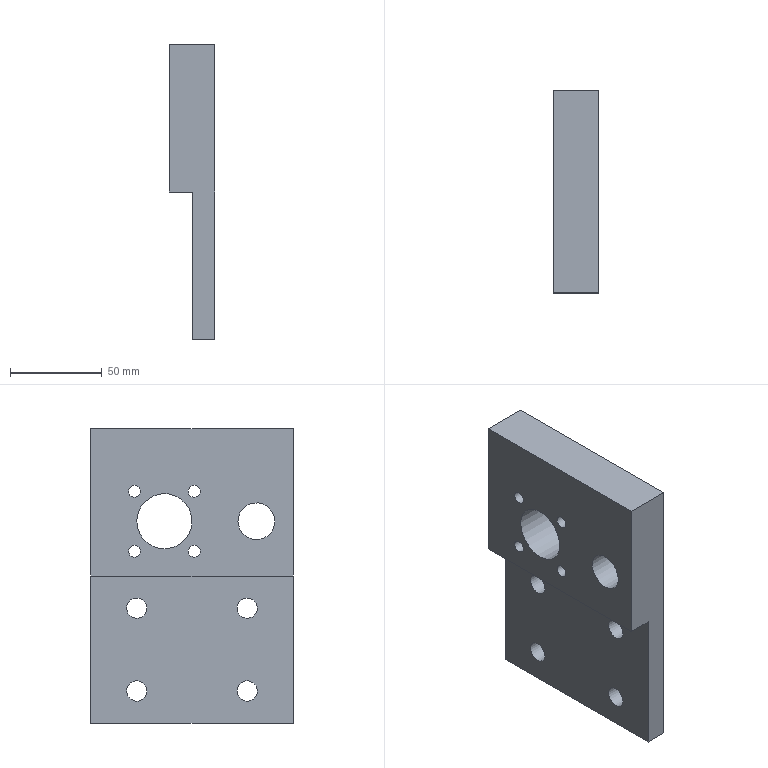Part | STEP file | SN10_015_002_PLACA | 1 solid | 18 faces | box 25 x 110 x 160 mm | volume 292195 mm3 | cylinder 10 | plane 8 | commonest cylinder face diameters 6.5 x4 11 x4 20 x1 30 x1
STEP:
#1=CARTESIAN_POINT('',(0.,0.,0.));
#2=DIRECTION('',(0.,0.,1.));
#3=DIRECTION('',(1.,0.,0.));
#4=AXIS2_PLACEMENT_3D('',#1,#2,#3);
#5=CARTESIAN_POINT('',(5499.,-1590.274,24.863));
#6=VERTEX_POINT('',#5);
#7=CARTESIAN_POINT('',(5499.,-1595.101,27.5));
#8=DIRECTION('',(-1.,0.,0.));
#9=DIRECTION('',(0.,1.,0.));
#10=AXIS2_PLACEMENT_3D('',#7,#8,#9);
#11=CIRCLE('',#10,5.5);
#12=CARTESIAN_POINT('',(5498.9,-1595.101,27.5));
#13=DIRECTION('',(-1.,0.,0.));
#14=DIRECTION('',(0.,0.8776,-0.4794));
#15=AXIS2_PLACEMENT_3D('',#12,#13,#14);
#16=CYLINDRICAL_SURFACE('',#15,5.5);
#17=CARTESIAN_POINT('',(-0.5,-0.1));
#18=DIRECTION('',(1.,0.));
#19=VECTOR('',#18,1.);
#20=LINE('',#17,#19);
#21=(GEOMETRIC_REPRESENTATION_CONTEXT(2)PARAMETRIC_REPRESENTATION_CONTEXT()REPRESENTATION_CONTEXT('',''));
#22=DEFINITIONAL_REPRESENTATION('',(#20),#21);
#23=PCURVE('',#16,#22);
#24=CARTESIAN_POINT('',(5499.,0.,0.));
#25=DIRECTION('',(1.,0.,0.));
#26=DIRECTION('',(0.,0.,-1.));
#27=AXIS2_PLACEMENT_3D('',#24,#25,#26);
#28=PLANE('',#27);
#29=CARTESIAN_POINT('',(-27.5,-1589.601));
#30=CARTESIAN_POINT('',(-17.974,-1589.601));
#31=CARTESIAN_POINT('',(-22.737,-1597.851));
#32=CARTESIAN_POINT('',(-27.5,-1606.101));
#33=CARTESIAN_POINT('',(-32.263,-1597.851));
#34=CARTESIAN_POINT('',(-37.026,-1589.601));
#35=CARTESIAN_POINT('',(-27.5,-1589.601));
#36=(BOUNDED_CURVE()B_SPLINE_CURVE(2,(#29,#30,#31,#32,#33,#34,#35),.UNSPECIFIED.,.T.,.F.)B_SPLINE_CURVE_WITH_KNOTS((1,2,2,2,2,1),(-2.094,0.,2.094,4.189,6.283,8.378),.UNSPECIFIED.)CURVE()GEOMETRIC_REPRESENTATION_ITEM()RATIONAL_B_SPLINE_CURVE((1.,0.5,1.,0.5,1.,0.5,1.))REPRESENTATION_ITEM(''));
#37=(GEOMETRIC_REPRESENTATION_CONTEXT(2)PARAMETRIC_REPRESENTATION_CONTEXT()REPRESENTATION_CONTEXT('',''));
#38=DEFINITIONAL_REPRESENTATION('',(#36),#37);
#39=PCURVE('',#28,#38);
#40=SURFACE_CURVE('',#11,(#23,#39),.PCURVE_S1.);
#41=EDGE_CURVE('',#6,#6,#40,.T.);
#42=ORIENTED_EDGE('',*,*,#41,.T.);
#43=CARTESIAN_POINT('',(5487.,-1590.274,24.863));
#44=VERTEX_POINT('',#43);
#45=CARTESIAN_POINT('',(5499.,-1590.274,24.863));
#46=CARTESIAN_POINT('',(5487.,-1590.274,24.863));
#47=B_SPLINE_CURVE_WITH_KNOTS('',1,(#45,#46),.UNSPECIFIED.,.F.,.F.,(2,2),(-0.1,11.9),.PIECEWISE_BEZIER_KNOTS.);
#48=CARTESIAN_POINT('',(6.283,0.));
#49=DIRECTION('',(0.,1.));
#50=VECTOR('',#49,1.);
#51=LINE('',#48,#50);
#52=(GEOMETRIC_REPRESENTATION_CONTEXT(2)PARAMETRIC_REPRESENTATION_CONTEXT()REPRESENTATION_CONTEXT('',''));
#53=DEFINITIONAL_REPRESENTATION('',(#51),#52);
#54=PCURVE('',#16,#53);
#55=CARTESIAN_POINT('',(0.,0.));
#56=DIRECTION('',(0.,1.));
#57=VECTOR('',#56,1.);
#58=LINE('',#55,#57);
#59=(GEOMETRIC_REPRESENTATION_CONTEXT(2)PARAMETRIC_REPRESENTATION_CONTEXT()REPRESENTATION_CONTEXT('',''));
#60=DEFINITIONAL_REPRESENTATION('',(#58),#59);
#61=PCURVE('',#16,#60);
#62=SEAM_CURVE('',#47,(#54,#61),.PCURVE_S1.);
#63=EDGE_CURVE('',#6,#44,#62,.T.);
#64=ORIENTED_EDGE('',*,*,#63,.T.);
#65=CARTESIAN_POINT('',(5487.,-1595.101,27.5));
#66=DIRECTION('',(-1.,0.,0.));
#67=DIRECTION('',(0.,1.,0.));
#68=AXIS2_PLACEMENT_3D('',#65,#66,#67);
#69=CIRCLE('',#68,5.5);
#70=CARTESIAN_POINT('',(-0.5,11.9));
#71=DIRECTION('',(1.,0.));
#72=VECTOR('',#71,1.);
#73=LINE('',#70,#72);
#74=(GEOMETRIC_REPRESENTATION_CONTEXT(2)PARAMETRIC_REPRESENTATION_CONTEXT()REPRESENTATION_CONTEXT('',''));
#75=DEFINITIONAL_REPRESENTATION('',(#73),#74);
#76=PCURVE('',#16,#75);
#77=CARTESIAN_POINT('',(5487.,-1620.101,45.));
#78=DIRECTION('',(1.,0.,0.));
#79=DIRECTION('',(0.,0.,-1.));
#80=AXIS2_PLACEMENT_3D('',#77,#78,#79);
#81=PLANE('',#80);
#82=CARTESIAN_POINT('',(17.5,30.5));
#83=CARTESIAN_POINT('',(27.026,30.5));
#84=CARTESIAN_POINT('',(22.263,22.25));
#85=CARTESIAN_POINT('',(17.5,14.));
#86=CARTESIAN_POINT('',(12.737,22.25));
#87=CARTESIAN_POINT('',(7.974,30.5));
#88=CARTESIAN_POINT('',(17.5,30.5));
#89=(BOUNDED_CURVE()B_SPLINE_CURVE(2,(#82,#83,#84,#85,#86,#87,#88),.UNSPECIFIED.,.T.,.F.)B_SPLINE_CURVE_WITH_KNOTS((1,2,2,2,2,1),(-2.094,0.,2.094,4.189,6.283,8.378),.UNSPECIFIED.)CURVE()GEOMETRIC_REPRESENTATION_ITEM()RATIONAL_B_SPLINE_CURVE((1.,0.5,1.,0.5,1.,0.5,1.))REPRESENTATION_ITEM(''));
#90=(GEOMETRIC_REPRESENTATION_CONTEXT(2)PARAMETRIC_REPRESENTATION_CONTEXT()REPRESENTATION_CONTEXT('',''));
#91=DEFINITIONAL_REPRESENTATION('',(#89),#90);
#92=PCURVE('',#81,#91);
#93=SURFACE_CURVE('',#69,(#76,#92),.PCURVE_S1.);
#94=EDGE_CURVE('',#44,#44,#93,.T.);
#95=ORIENTED_EDGE('',*,*,#94,.F.);
#96=ORIENTED_EDGE('',*,*,#63,.F.);
#97=EDGE_LOOP('',(#42,#64,#95,#96));
#98=FACE_BOUND('',#97,.F.);
#99=ADVANCED_FACE('',(#98),#16,.F.);
#100=CARTESIAN_POINT('',(5487.,-1620.101,-35.));
#101=VERTEX_POINT('',#100);
#102=CARTESIAN_POINT('',(5499.,-1620.101,-35.));
#103=VERTEX_POINT('',#102);
#104=CARTESIAN_POINT('',(5487.,-1620.101,-35.));
#105=DIRECTION('',(1.,0.,0.));
#106=VECTOR('',#105,1.);
#107=LINE('',#104,#106);
#108=CARTESIAN_POINT('',(5487.,-1510.101,-35.));
#109=DIRECTION('',(0.,0.,1.));
#110=DIRECTION('',(1.,0.,0.));
#111=AXIS2_PLACEMENT_3D('',#108,#109,#110);
#112=PLANE('',#111);
#113=CARTESIAN_POINT('',(0.,-110.));
#114=DIRECTION('',(1.,0.));
#115=VECTOR('',#114,1.);
#116=LINE('',#113,#115);
#117=(GEOMETRIC_REPRESENTATION_CONTEXT(2)PARAMETRIC_REPRESENTATION_CONTEXT()REPRESENTATION_CONTEXT('',''));
#118=DEFINITIONAL_REPRESENTATION('',(#116),#117);
#119=PCURVE('',#112,#118);
#120=CARTESIAN_POINT('',(5487.,-1620.101,45.));
#121=DIRECTION('',(0.,1.,0.));
#122=DIRECTION('',(0.,0.,1.));
#123=AXIS2_PLACEMENT_3D('',#120,#121,#122);
#124=PLANE('',#123);
#125=CARTESIAN_POINT('',(-80.,0.));
#126=DIRECTION('',(0.,1.));
#127=VECTOR('',#126,1.);
#128=LINE('',#125,#127);
#129=(GEOMETRIC_REPRESENTATION_CONTEXT(2)PARAMETRIC_REPRESENTATION_CONTEXT()REPRESENTATION_CONTEXT('',''));
#130=DEFINITIONAL_REPRESENTATION('',(#128),#129);
#131=PCURVE('',#124,#130);
#132=SURFACE_CURVE('',#107,(#119,#131),.PCURVE_S1.);
#133=EDGE_CURVE('',#101,#103,#132,.T.);
#134=ORIENTED_EDGE('',*,*,#133,.F.);
#135=CARTESIAN_POINT('',(5487.,-1510.101,-35.));
#136=VERTEX_POINT('',#135);
#137=CARTESIAN_POINT('',(5487.,-1510.101,-35.));
#138=DIRECTION('',(0.,-1.,0.));
#139=VECTOR('',#138,1.);
#140=LINE('',#137,#139);
#141=CARTESIAN_POINT('',(0.,0.));
#142=DIRECTION('',(0.,-1.));
#143=VECTOR('',#142,1.);
#144=LINE('',#141,#143);
#145=(GEOMETRIC_REPRESENTATION_CONTEXT(2)PARAMETRIC_REPRESENTATION_CONTEXT()REPRESENTATION_CONTEXT('',''));
#146=DEFINITIONAL_REPRESENTATION('',(#144),#145);
#147=PCURVE('',#112,#146);
#148=CARTESIAN_POINT('',(80.,110.));
#149=DIRECTION('',(0.,-1.));
#150=VECTOR('',#149,1.);
#151=LINE('',#148,#150);
#152=(GEOMETRIC_REPRESENTATION_CONTEXT(2)PARAMETRIC_REPRESENTATION_CONTEXT()REPRESENTATION_CONTEXT('',''));
#153=DEFINITIONAL_REPRESENTATION('',(#151),#152);
#154=PCURVE('',#81,#153);
#155=SURFACE_CURVE('',#140,(#147,#154),.PCURVE_S1.);
#156=EDGE_CURVE('',#136,#101,#155,.T.);
#157=ORIENTED_EDGE('',*,*,#156,.F.);
#158=CARTESIAN_POINT('',(5499.,-1510.101,-35.));
#159=VERTEX_POINT('',#158);
#160=CARTESIAN_POINT('',(5487.,-1510.101,-35.));
#161=DIRECTION('',(1.,0.,0.));
#162=VECTOR('',#161,1.);
#163=LINE('',#160,#162);
#164=CARTESIAN_POINT('',(0.,0.));
#165=DIRECTION('',(1.,0.));
#166=VECTOR('',#165,1.);
#167=LINE('',#164,#166);
#168=(GEOMETRIC_REPRESENTATION_CONTEXT(2)PARAMETRIC_REPRESENTATION_CONTEXT()REPRESENTATION_CONTEXT('',''));
#169=DEFINITIONAL_REPRESENTATION('',(#167),#168);
#170=PCURVE('',#112,#169);
#171=CARTESIAN_POINT('',(5473.6,-1510.101,45.));
#172=DIRECTION('',(0.,-1.,0.));
#173=DIRECTION('',(0.,0.,-1.));
#174=AXIS2_PLACEMENT_3D('',#171,#172,#173);
#175=PLANE('',#174);
#176=CARTESIAN_POINT('',(80.,13.4));
#177=DIRECTION('',(0.,1.));
#178=VECTOR('',#177,1.);
#179=LINE('',#176,#178);
#180=(GEOMETRIC_REPRESENTATION_CONTEXT(2)PARAMETRIC_REPRESENTATION_CONTEXT()REPRESENTATION_CONTEXT('',''));
#181=DEFINITIONAL_REPRESENTATION('',(#179),#180);
#182=PCURVE('',#175,#181);
#183=SURFACE_CURVE('',#163,(#170,#182),.PCURVE_S1.);
#184=EDGE_CURVE('',#136,#159,#183,.T.);
#185=ORIENTED_EDGE('',*,*,#184,.T.);
#186=CARTESIAN_POINT('',(5499.,-1510.101,-35.));
#187=DIRECTION('',(0.,-1.,0.));
#188=VECTOR('',#187,1.);
#189=LINE('',#186,#188);
#190=CARTESIAN_POINT('',(12.,0.));
#191=DIRECTION('',(0.,-1.));
#192=VECTOR('',#191,1.);
#193=LINE('',#190,#192);
#194=(GEOMETRIC_REPRESENTATION_CONTEXT(2)PARAMETRIC_REPRESENTATION_CONTEXT()REPRESENTATION_CONTEXT('',''));
#195=DEFINITIONAL_REPRESENTATION('',(#193),#194);
#196=PCURVE('',#112,#195);
#197=CARTESIAN_POINT('',(35.,-1510.101));
#198=DIRECTION('',(0.,-1.));
#199=VECTOR('',#198,1.);
#200=LINE('',#197,#199);
#201=(GEOMETRIC_REPRESENTATION_CONTEXT(2)PARAMETRIC_REPRESENTATION_CONTEXT()REPRESENTATION_CONTEXT('',''));
#202=DEFINITIONAL_REPRESENTATION('',(#200),#201);
#203=PCURVE('',#28,#202);
#204=SURFACE_CURVE('',#189,(#196,#203),.PCURVE_S1.);
#205=EDGE_CURVE('',#159,#103,#204,.T.);
#206=ORIENTED_EDGE('',*,*,#205,.T.);
#207=EDGE_LOOP('',(#134,#157,#185,#206));
#208=FACE_BOUND('',#207,.T.);
#209=ADVANCED_FACE('',(#208),#112,.F.);
#210=CARTESIAN_POINT('',(5487.,-1620.101,45.));
#211=VERTEX_POINT('',#210);
#212=CARTESIAN_POINT('',(5487.,-1510.101,45.));
#213=VERTEX_POINT('',#212);
#214=CARTESIAN_POINT('',(5487.,-1620.101,45.));
#215=DIRECTION('',(0.,1.,0.));
#216=VECTOR('',#215,1.);
#217=LINE('',#214,#216);
#218=CARTESIAN_POINT('',(0.,0.));
#219=DIRECTION('',(0.,1.));
#220=VECTOR('',#219,1.);
#221=LINE('',#218,#220);
#222=(GEOMETRIC_REPRESENTATION_CONTEXT(2)PARAMETRIC_REPRESENTATION_CONTEXT()REPRESENTATION_CONTEXT('',''));
#223=DEFINITIONAL_REPRESENTATION('',(#221),#222);
#224=PCURVE('',#81,#223);
#225=CARTESIAN_POINT('',(0.,0.,45.));
#226=DIRECTION('',(0.,0.,1.));
#227=DIRECTION('',(1.,0.,0.));
#228=AXIS2_PLACEMENT_3D('',#225,#226,#227);
#229=PLANE('',#228);
#230=CARTESIAN_POINT('',(5487.,-1620.101));
#231=DIRECTION('',(0.,1.));
#232=VECTOR('',#231,1.);
#233=LINE('',#230,#232);
#234=(GEOMETRIC_REPRESENTATION_CONTEXT(2)PARAMETRIC_REPRESENTATION_CONTEXT()REPRESENTATION_CONTEXT('',''));
#235=DEFINITIONAL_REPRESENTATION('',(#233),#234);
#236=PCURVE('',#229,#235);
#237=SURFACE_CURVE('',#217,(#224,#236),.PCURVE_S1.);
#238=EDGE_CURVE('',#211,#213,#237,.T.);
#239=ORIENTED_EDGE('',*,*,#238,.T.);
#240=CARTESIAN_POINT('',(5487.,-1510.101,-35.));
#241=DIRECTION('',(0.,0.,1.));
#242=VECTOR('',#241,1.);
#243=LINE('',#240,#242);
#244=CARTESIAN_POINT('',(80.,110.));
#245=DIRECTION('',(-1.,0.));
#246=VECTOR('',#245,1.);
#247=LINE('',#244,#246);
#248=(GEOMETRIC_REPRESENTATION_CONTEXT(2)PARAMETRIC_REPRESENTATION_CONTEXT()REPRESENTATION_CONTEXT('',''));
#249=DEFINITIONAL_REPRESENTATION('',(#247),#248);
#250=PCURVE('',#81,#249);
#251=CARTESIAN_POINT('',(80.,13.4));
#252=DIRECTION('',(-1.,0.));
#253=VECTOR('',#252,1.);
#254=LINE('',#251,#253);
#255=(GEOMETRIC_REPRESENTATION_CONTEXT(2)PARAMETRIC_REPRESENTATION_CONTEXT()REPRESENTATION_CONTEXT('',''));
#256=DEFINITIONAL_REPRESENTATION('',(#254),#255);
#257=PCURVE('',#175,#256);
#258=SURFACE_CURVE('',#243,(#250,#257),.PCURVE_S1.);
#259=EDGE_CURVE('',#136,#213,#258,.T.);
#260=ORIENTED_EDGE('',*,*,#259,.F.);
#261=ORIENTED_EDGE('',*,*,#156,.T.);
#262=CARTESIAN_POINT('',(5487.,-1620.101,45.));
#263=DIRECTION('',(0.,0.,-1.));
#264=VECTOR('',#263,1.);
#265=LINE('',#262,#264);
#266=CARTESIAN_POINT('',(0.,0.));
#267=DIRECTION('',(1.,0.));
#268=VECTOR('',#267,1.);
#269=LINE('',#266,#268);
#270=(GEOMETRIC_REPRESENTATION_CONTEXT(2)PARAMETRIC_REPRESENTATION_CONTEXT()REPRESENTATION_CONTEXT('',''));
#271=DEFINITIONAL_REPRESENTATION('',(#269),#270);
#272=PCURVE('',#81,#271);
#273=CARTESIAN_POINT('',(0.,0.));
#274=DIRECTION('',(-1.,0.));
#275=VECTOR('',#274,1.);
#276=LINE('',#273,#275);
#277=(GEOMETRIC_REPRESENTATION_CONTEXT(2)PARAMETRIC_REPRESENTATION_CONTEXT()REPRESENTATION_CONTEXT('',''));
#278=DEFINITIONAL_REPRESENTATION('',(#276),#277);
#279=PCURVE('',#124,#278);
#280=SURFACE_CURVE('',#265,(#272,#279),.PCURVE_S1.);
#281=EDGE_CURVE('',#211,#101,#280,.T.);
#282=ORIENTED_EDGE('',*,*,#281,.F.);
#283=EDGE_LOOP('',(#239,#260,#261,#282));
#284=FACE_BOUND('',#283,.T.);
#285=ORIENTED_EDGE('',*,*,#94,.F.);
#286=EDGE_LOOP('',(#285));
#287=FACE_BOUND('',#286,.T.);
#288=CARTESIAN_POINT('',(5487.,-1530.274,24.863));
#289=VERTEX_POINT('',#288);
#290=CARTESIAN_POINT('',(5487.,-1535.101,27.5));
#291=DIRECTION('',(1.,0.,0.));
#292=DIRECTION('',(0.,1.,0.));
#293=AXIS2_PLACEMENT_3D('',#290,#291,#292);
#294=CIRCLE('',#293,5.5);
#295=CARTESIAN_POINT('',(17.5,85.));
#296=DIRECTION('',(0.,1.));
#297=AXIS2_PLACEMENT_2D('',#295,#296);
#298=CIRCLE('',#297,5.5);
#299=(GEOMETRIC_REPRESENTATION_CONTEXT(2)PARAMETRIC_REPRESENTATION_CONTEXT()REPRESENTATION_CONTEXT('',''));
#300=DEFINITIONAL_REPRESENTATION('',(#298),#299);
#301=PCURVE('',#81,#300);
#302=CARTESIAN_POINT('',(5498.9,-1535.101,27.5));
#303=DIRECTION('',(-1.,0.,0.));
#304=DIRECTION('',(0.,0.8776,-0.4794));
#305=AXIS2_PLACEMENT_3D('',#302,#303,#304);
#306=CYLINDRICAL_SURFACE('',#305,5.5);
#307=CARTESIAN_POINT('',(12.066,11.9));
#308=DIRECTION('',(-1.,0.));
#309=VECTOR('',#308,1.);
#310=LINE('',#307,#309);
#311=(GEOMETRIC_REPRESENTATION_CONTEXT(2)PARAMETRIC_REPRESENTATION_CONTEXT()REPRESENTATION_CONTEXT('',''));
#312=DEFINITIONAL_REPRESENTATION('',(#310),#311);
#313=PCURVE('',#306,#312);
#314=SURFACE_CURVE('',#294,(#301,#313),.PCURVE_S1.);
#315=EDGE_CURVE('',#289,#289,#314,.T.);
#316=ORIENTED_EDGE('',*,*,#315,.T.);
#317=EDGE_LOOP('',(#316));
#318=FACE_BOUND('',#317,.T.);
#319=CARTESIAN_POINT('',(5487.,-1590.274,-20.137));
#320=VERTEX_POINT('',#319);
#321=CARTESIAN_POINT('',(5487.,-1595.101,-17.5));
#322=DIRECTION('',(1.,0.,0.));
#323=DIRECTION('',(0.,1.,0.));
#324=AXIS2_PLACEMENT_3D('',#321,#322,#323);
#325=CIRCLE('',#324,5.5);
#326=CARTESIAN_POINT('',(62.5,25.));
#327=DIRECTION('',(0.,1.));
#328=AXIS2_PLACEMENT_2D('',#326,#327);
#329=CIRCLE('',#328,5.5);
#330=(GEOMETRIC_REPRESENTATION_CONTEXT(2)PARAMETRIC_REPRESENTATION_CONTEXT()REPRESENTATION_CONTEXT('',''));
#331=DEFINITIONAL_REPRESENTATION('',(#329),#330);
#332=PCURVE('',#81,#331);
#333=CARTESIAN_POINT('',(5498.9,-1595.101,-17.5));
#334=DIRECTION('',(-1.,0.,0.));
#335=DIRECTION('',(0.,0.8776,-0.4794));
#336=AXIS2_PLACEMENT_3D('',#333,#334,#335);
#337=CYLINDRICAL_SURFACE('',#336,5.5);
#338=CARTESIAN_POINT('',(12.066,11.9));
#339=DIRECTION('',(-1.,0.));
#340=VECTOR('',#339,1.);
#341=LINE('',#338,#340);
#342=(GEOMETRIC_REPRESENTATION_CONTEXT(2)PARAMETRIC_REPRESENTATION_CONTEXT()REPRESENTATION_CONTEXT('',''));
#343=DEFINITIONAL_REPRESENTATION('',(#341),#342);
#344=PCURVE('',#337,#343);
#345=SURFACE_CURVE('',#325,(#332,#344),.PCURVE_S1.);
#346=EDGE_CURVE('',#320,#320,#345,.T.);
#347=ORIENTED_EDGE('',*,*,#346,.T.);
#348=EDGE_LOOP('',(#347));
#349=FACE_BOUND('',#348,.T.);
#350=CARTESIAN_POINT('',(5487.,-1530.274,-20.137));
#351=VERTEX_POINT('',#350);
#352=CARTESIAN_POINT('',(5487.,-1535.101,-17.5));
#353=DIRECTION('',(1.,0.,0.));
#354=DIRECTION('',(0.,1.,0.));
#355=AXIS2_PLACEMENT_3D('',#352,#353,#354);
#356=CIRCLE('',#355,5.5);
#357=CARTESIAN_POINT('',(62.5,85.));
#358=DIRECTION('',(0.,1.));
#359=AXIS2_PLACEMENT_2D('',#357,#358);
#360=CIRCLE('',#359,5.5);
#361=(GEOMETRIC_REPRESENTATION_CONTEXT(2)PARAMETRIC_REPRESENTATION_CONTEXT()REPRESENTATION_CONTEXT('',''));
#362=DEFINITIONAL_REPRESENTATION('',(#360),#361);
#363=PCURVE('',#81,#362);
#364=CARTESIAN_POINT('',(5498.9,-1535.101,-17.5));
#365=DIRECTION('',(-1.,0.,0.));
#366=DIRECTION('',(0.,0.8776,-0.4794));
#367=AXIS2_PLACEMENT_3D('',#364,#365,#366);
#368=CYLINDRICAL_SURFACE('',#367,5.5);
#369=CARTESIAN_POINT('',(12.066,11.9));
#370=DIRECTION('',(-1.,0.));
#371=VECTOR('',#370,1.);
#372=LINE('',#369,#371);
#373=(GEOMETRIC_REPRESENTATION_CONTEXT(2)PARAMETRIC_REPRESENTATION_CONTEXT()REPRESENTATION_CONTEXT('',''));
#374=DEFINITIONAL_REPRESENTATION('',(#372),#373);
#375=PCURVE('',#368,#374);
#376=SURFACE_CURVE('',#356,(#363,#375),.PCURVE_S1.);
#377=EDGE_CURVE('',#351,#351,#376,.T.);
#378=ORIENTED_EDGE('',*,*,#377,.T.);
#379=EDGE_LOOP('',(#378));
#380=FACE_BOUND('',#379,.T.);
#381=ADVANCED_FACE('',(#284,#287,#318,#349,#380),#81,.F.);
#382=CARTESIAN_POINT('',(5499.,-1620.101,125.));
#383=VERTEX_POINT('',#382);
#384=CARTESIAN_POINT('',(5499.,-1620.101,125.));
#385=DIRECTION('',(0.,0.,-1.));
#386=VECTOR('',#385,1.);
#387=LINE('',#384,#386);
#388=CARTESIAN_POINT('',(-125.,-1620.101));
#389=DIRECTION('',(1.,0.));
#390=VECTOR('',#389,1.);
#391=LINE('',#388,#390);
#392=(GEOMETRIC_REPRESENTATION_CONTEXT(2)PARAMETRIC_REPRESENTATION_CONTEXT()REPRESENTATION_CONTEXT('',''));
#393=DEFINITIONAL_REPRESENTATION('',(#391),#392);
#394=PCURVE('',#28,#393);
#395=CARTESIAN_POINT('',(80.,12.));
#396=DIRECTION('',(-1.,0.));
#397=VECTOR('',#396,1.);
#398=LINE('',#395,#397);
#399=(GEOMETRIC_REPRESENTATION_CONTEXT(2)PARAMETRIC_REPRESENTATION_CONTEXT()REPRESENTATION_CONTEXT('',''));
#400=DEFINITIONAL_REPRESENTATION('',(#398),#399);
#401=PCURVE('',#124,#400);
#402=SURFACE_CURVE('',#387,(#394,#401),.PCURVE_S1.);
#403=EDGE_CURVE('',#383,#103,#402,.T.);
#404=ORIENTED_EDGE('',*,*,#403,.T.);
#405=ORIENTED_EDGE('',*,*,#205,.F.);
#406=CARTESIAN_POINT('',(5499.,-1510.101,125.));
#407=VERTEX_POINT('',#406);
#408=CARTESIAN_POINT('',(5499.,-1510.101,-35.));
#409=DIRECTION('',(0.,0.,1.));
#410=VECTOR('',#409,1.);
#411=LINE('',#408,#410);
#412=CARTESIAN_POINT('',(35.,-1510.101));
#413=DIRECTION('',(-1.,0.));
#414=VECTOR('',#413,1.);
#415=LINE('',#412,#414);
#416=(GEOMETRIC_REPRESENTATION_CONTEXT(2)PARAMETRIC_REPRESENTATION_CONTEXT()REPRESENTATION_CONTEXT('',''));
#417=DEFINITIONAL_REPRESENTATION('',(#415),#416);
#418=PCURVE('',#28,#417);
#419=CARTESIAN_POINT('',(80.,25.4));
#420=DIRECTION('',(-1.,0.));
#421=VECTOR('',#420,1.);
#422=LINE('',#419,#421);
#423=(GEOMETRIC_REPRESENTATION_CONTEXT(2)PARAMETRIC_REPRESENTATION_CONTEXT()REPRESENTATION_CONTEXT('',''));
#424=DEFINITIONAL_REPRESENTATION('',(#422),#423);
#425=PCURVE('',#175,#424);
#426=SURFACE_CURVE('',#411,(#418,#425),.PCURVE_S1.);
#427=EDGE_CURVE('',#159,#407,#426,.T.);
#428=ORIENTED_EDGE('',*,*,#427,.T.);
#429=CARTESIAN_POINT('',(5499.,-1620.101,125.));
#430=DIRECTION('',(0.,1.,0.));
#431=VECTOR('',#430,1.);
#432=LINE('',#429,#431);
#433=CARTESIAN_POINT('',(-125.,-1620.101));
#434=DIRECTION('',(0.,1.));
#435=VECTOR('',#434,1.);
#436=LINE('',#433,#435);
#437=(GEOMETRIC_REPRESENTATION_CONTEXT(2)PARAMETRIC_REPRESENTATION_CONTEXT()REPRESENTATION_CONTEXT('',''));
#438=DEFINITIONAL_REPRESENTATION('',(#436),#437);
#439=PCURVE('',#28,#438);
#440=CARTESIAN_POINT('',(0.,0.,125.));
#441=DIRECTION('',(0.,0.,1.));
#442=DIRECTION('',(1.,0.,0.));
#443=AXIS2_PLACEMENT_3D('',#440,#441,#442);
#444=PLANE('',#443);
#445=CARTESIAN_POINT('',(5499.,-1620.101));
#446=DIRECTION('',(0.,1.));
#447=VECTOR('',#446,1.);
#448=LINE('',#445,#447);
#449=(GEOMETRIC_REPRESENTATION_CONTEXT(2)PARAMETRIC_REPRESENTATION_CONTEXT()REPRESENTATION_CONTEXT('',''));
#450=DEFINITIONAL_REPRESENTATION('',(#448),#449);
#451=PCURVE('',#444,#450);
#452=SURFACE_CURVE('',#432,(#439,#451),.PCURVE_S1.);
#453=EDGE_CURVE('',#383,#407,#452,.T.);
#454=ORIENTED_EDGE('',*,*,#453,.F.);
#455=EDGE_LOOP('',(#404,#405,#428,#454));
#456=FACE_BOUND('',#455,.T.);
#457=ORIENTED_EDGE('',*,*,#41,.T.);
#458=EDGE_LOOP('',(#457));
#459=FACE_BOUND('',#458,.T.);
#460=CARTESIAN_POINT('',(5499.,-1591.325,69.956));
#461=VERTEX_POINT('',#460);
#462=CARTESIAN_POINT('',(5499.,-1600.101,74.75));
#463=DIRECTION('',(1.,0.,0.));
#464=DIRECTION('',(0.,1.,0.));
#465=AXIS2_PLACEMENT_3D('',#462,#463,#464);
#466=CIRCLE('',#465,10.);
#467=CARTESIAN_POINT('',(-74.75,-1600.101));
#468=DIRECTION('',(0.,1.));
#469=AXIS2_PLACEMENT_2D('',#467,#468);
#470=CIRCLE('',#469,10.);
#471=(GEOMETRIC_REPRESENTATION_CONTEXT(2)PARAMETRIC_REPRESENTATION_CONTEXT()REPRESENTATION_CONTEXT('',''));
#472=DEFINITIONAL_REPRESENTATION('',(#470),#471);
#473=PCURVE('',#28,#472);
#474=CARTESIAN_POINT('',(5498.9,-1600.101,74.75));
#475=DIRECTION('',(-1.,0.,0.));
#476=DIRECTION('',(0.,0.8776,-0.4794));
#477=AXIS2_PLACEMENT_3D('',#474,#475,#476);
#478=CYLINDRICAL_SURFACE('',#477,10.);
#479=CARTESIAN_POINT('',(12.066,-0.1));
#480=DIRECTION('',(-1.,0.));
#481=VECTOR('',#480,1.);
#482=LINE('',#479,#481);
#483=(GEOMETRIC_REPRESENTATION_CONTEXT(2)PARAMETRIC_REPRESENTATION_CONTEXT()REPRESENTATION_CONTEXT('',''));
#484=DEFINITIONAL_REPRESENTATION('',(#482),#483);
#485=PCURVE('',#478,#484);
#486=SURFACE_CURVE('',#466,(#473,#485),.PCURVE_S1.);
#487=EDGE_CURVE('',#461,#461,#486,.T.);
#488=ORIENTED_EDGE('',*,*,#487,.F.);
#489=EDGE_LOOP('',(#488));
#490=FACE_BOUND('',#489,.T.);
#491=CARTESIAN_POINT('',(5499.,-1569.203,89.442));
#492=VERTEX_POINT('',#491);
#493=CARTESIAN_POINT('',(5499.,-1566.351,91.));
#494=DIRECTION('',(1.,0.,0.));
#495=DIRECTION('',(0.,1.,0.));
#496=AXIS2_PLACEMENT_3D('',#493,#494,#495);
#497=CIRCLE('',#496,3.25);
#498=CARTESIAN_POINT('',(-91.,-1566.351));
#499=DIRECTION('',(0.,1.));
#500=AXIS2_PLACEMENT_2D('',#498,#499);
#501=CIRCLE('',#500,3.25);
#502=(GEOMETRIC_REPRESENTATION_CONTEXT(2)PARAMETRIC_REPRESENTATION_CONTEXT()REPRESENTATION_CONTEXT('',''));
#503=DEFINITIONAL_REPRESENTATION('',(#501),#502);
#504=PCURVE('',#28,#503);
#505=CARTESIAN_POINT('',(5473.7,-1566.351,91.));
#506=DIRECTION('',(1.,0.,0.));
#507=DIRECTION('',(0.,0.8776,0.4794));
#508=AXIS2_PLACEMENT_3D('',#505,#506,#507);
#509=CYLINDRICAL_SURFACE('',#508,3.25);
#510=CARTESIAN_POINT('',(-0.5,25.3));
#511=DIRECTION('',(1.,0.));
#512=VECTOR('',#511,1.);
#513=LINE('',#510,#512);
#514=(GEOMETRIC_REPRESENTATION_CONTEXT(2)PARAMETRIC_REPRESENTATION_CONTEXT()REPRESENTATION_CONTEXT('',''));
#515=DEFINITIONAL_REPRESENTATION('',(#513),#514);
#516=PCURVE('',#509,#515);
#517=SURFACE_CURVE('',#497,(#504,#516),.PCURVE_S1.);
#518=EDGE_CURVE('',#492,#492,#517,.T.);
#519=ORIENTED_EDGE('',*,*,#518,.F.);
#520=EDGE_LOOP('',(#519));
#521=FACE_BOUND('',#520,.T.);
#522=CARTESIAN_POINT('',(5499.,-1563.264,67.559));
#523=VERTEX_POINT('',#522);
#524=CARTESIAN_POINT('',(5499.,-1550.101,74.75));
#525=DIRECTION('',(1.,0.,0.));
#526=DIRECTION('',(0.,1.,0.));
#527=AXIS2_PLACEMENT_3D('',#524,#525,#526);
#528=CIRCLE('',#527,15.);
#529=CARTESIAN_POINT('',(-74.75,-1550.101));
#530=DIRECTION('',(0.,1.));
#531=AXIS2_PLACEMENT_2D('',#529,#530);
#532=CIRCLE('',#531,15.);
#533=(GEOMETRIC_REPRESENTATION_CONTEXT(2)PARAMETRIC_REPRESENTATION_CONTEXT()REPRESENTATION_CONTEXT('',''));
#534=DEFINITIONAL_REPRESENTATION('',(#532),#533);
#535=PCURVE('',#28,#534);
#536=CARTESIAN_POINT('',(5473.7,-1550.101,74.75));
#537=DIRECTION('',(1.,0.,0.));
#538=DIRECTION('',(0.,0.8776,0.4794));
#539=AXIS2_PLACEMENT_3D('',#536,#537,#538);
#540=CYLINDRICAL_SURFACE('',#539,15.);
#541=CARTESIAN_POINT('',(-0.5,25.3));
#542=DIRECTION('',(1.,0.));
#543=VECTOR('',#542,1.);
#544=LINE('',#541,#543);
#545=(GEOMETRIC_REPRESENTATION_CONTEXT(2)PARAMETRIC_REPRESENTATION_CONTEXT()REPRESENTATION_CONTEXT('',''));
#546=DEFINITIONAL_REPRESENTATION('',(#544),#545);
#547=PCURVE('',#540,#546);
#548=SURFACE_CURVE('',#528,(#535,#547),.PCURVE_S1.);
#549=EDGE_CURVE('',#523,#523,#548,.T.);
#550=ORIENTED_EDGE('',*,*,#549,.F.);
#551=EDGE_LOOP('',(#550));
#552=FACE_BOUND('',#551,.T.);
#553=CARTESIAN_POINT('',(5499.,-1530.998,92.558));
#554=VERTEX_POINT('',#553);
#555=CARTESIAN_POINT('',(5499.,-1533.851,91.));
#556=DIRECTION('',(1.,0.,0.));
#557=DIRECTION('',(0.,1.,0.));
#558=AXIS2_PLACEMENT_3D('',#555,#556,#557);
#559=CIRCLE('',#558,3.25);
#560=CARTESIAN_POINT('',(-91.,-1533.851));
#561=DIRECTION('',(0.,1.));
#562=AXIS2_PLACEMENT_2D('',#560,#561);
#563=CIRCLE('',#562,3.25);
#564=(GEOMETRIC_REPRESENTATION_CONTEXT(2)PARAMETRIC_REPRESENTATION_CONTEXT()REPRESENTATION_CONTEXT('',''));
#565=DEFINITIONAL_REPRESENTATION('',(#563),#564);
#566=PCURVE('',#28,#565);
#567=CARTESIAN_POINT('',(5473.7,-1533.851,91.));
#568=DIRECTION('',(1.,0.,0.));
#569=DIRECTION('',(0.,0.8776,0.4794));
#570=AXIS2_PLACEMENT_3D('',#567,#568,#569);
#571=CYLINDRICAL_SURFACE('',#570,3.25);
#572=CARTESIAN_POINT('',(-0.5,25.3));
#573=DIRECTION('',(1.,0.));
#574=VECTOR('',#573,1.);
#575=LINE('',#572,#574);
#576=(GEOMETRIC_REPRESENTATION_CONTEXT(2)PARAMETRIC_REPRESENTATION_CONTEXT()REPRESENTATION_CONTEXT('',''));
#577=DEFINITIONAL_REPRESENTATION('',(#575),#576);
#578=PCURVE('',#571,#577);
#579=SURFACE_CURVE('',#559,(#566,#578),.PCURVE_S1.);
#580=EDGE_CURVE('',#554,#554,#579,.T.);
#581=ORIENTED_EDGE('',*,*,#580,.F.);
#582=EDGE_LOOP('',(#581));
#583=FACE_BOUND('',#582,.T.);
#584=CARTESIAN_POINT('',(5499.,-1563.498,60.058));
#585=VERTEX_POINT('',#584);
#586=CARTESIAN_POINT('',(5499.,-1566.351,58.5));
#587=DIRECTION('',(1.,0.,0.));
#588=DIRECTION('',(0.,1.,0.));
#589=AXIS2_PLACEMENT_3D('',#586,#587,#588);
#590=CIRCLE('',#589,3.25);
#591=CARTESIAN_POINT('',(-58.5,-1566.351));
#592=DIRECTION('',(0.,1.));
#593=AXIS2_PLACEMENT_2D('',#591,#592);
#594=CIRCLE('',#593,3.25);
#595=(GEOMETRIC_REPRESENTATION_CONTEXT(2)PARAMETRIC_REPRESENTATION_CONTEXT()REPRESENTATION_CONTEXT('',''));
#596=DEFINITIONAL_REPRESENTATION('',(#594),#595);
#597=PCURVE('',#28,#596);
#598=CARTESIAN_POINT('',(5473.7,-1566.351,58.5));
#599=DIRECTION('',(1.,0.,0.));
#600=DIRECTION('',(0.,0.8776,0.4794));
#601=AXIS2_PLACEMENT_3D('',#598,#599,#600);
#602=CYLINDRICAL_SURFACE('',#601,3.25);
#603=CARTESIAN_POINT('',(-0.5,25.3));
#604=DIRECTION('',(1.,0.));
#605=VECTOR('',#604,1.);
#606=LINE('',#603,#605);
#607=(GEOMETRIC_REPRESENTATION_CONTEXT(2)PARAMETRIC_REPRESENTATION_CONTEXT()REPRESENTATION_CONTEXT('',''));
#608=DEFINITIONAL_REPRESENTATION('',(#606),#607);
#609=PCURVE('',#602,#608);
#610=SURFACE_CURVE('',#590,(#597,#609),.PCURVE_S1.);
#611=EDGE_CURVE('',#585,#585,#610,.T.);
#612=ORIENTED_EDGE('',*,*,#611,.F.);
#613=EDGE_LOOP('',(#612));
#614=FACE_BOUND('',#613,.T.);
#615=CARTESIAN_POINT('',(5499.,-1530.998,60.058));
#616=VERTEX_POINT('',#615);
#617=CARTESIAN_POINT('',(5499.,-1533.851,58.5));
#618=DIRECTION('',(1.,0.,0.));
#619=DIRECTION('',(0.,1.,0.));
#620=AXIS2_PLACEMENT_3D('',#617,#618,#619);
#621=CIRCLE('',#620,3.25);
#622=CARTESIAN_POINT('',(-58.5,-1533.851));
#623=DIRECTION('',(0.,1.));
#624=AXIS2_PLACEMENT_2D('',#622,#623);
#625=CIRCLE('',#624,3.25);
#626=(GEOMETRIC_REPRESENTATION_CONTEXT(2)PARAMETRIC_REPRESENTATION_CONTEXT()REPRESENTATION_CONTEXT('',''));
#627=DEFINITIONAL_REPRESENTATION('',(#625),#626);
#628=PCURVE('',#28,#627);
#629=CARTESIAN_POINT('',(5473.7,-1533.851,58.5));
#630=DIRECTION('',(1.,0.,0.));
#631=DIRECTION('',(0.,0.8776,0.4794));
#632=AXIS2_PLACEMENT_3D('',#629,#630,#631);
#633=CYLINDRICAL_SURFACE('',#632,3.25);
#634=CARTESIAN_POINT('',(-0.5,25.3));
#635=DIRECTION('',(1.,0.));
#636=VECTOR('',#635,1.);
#637=LINE('',#634,#636);
#638=(GEOMETRIC_REPRESENTATION_CONTEXT(2)PARAMETRIC_REPRESENTATION_CONTEXT()REPRESENTATION_CONTEXT('',''));
#639=DEFINITIONAL_REPRESENTATION('',(#637),#638);
#640=PCURVE('',#633,#639);
#641=SURFACE_CURVE('',#621,(#628,#640),.PCURVE_S1.);
#642=EDGE_CURVE('',#616,#616,#641,.T.);
#643=ORIENTED_EDGE('',*,*,#642,.F.);
#644=EDGE_LOOP('',(#643));
#645=FACE_BOUND('',#644,.T.);
#646=CARTESIAN_POINT('',(5499.,-1530.274,24.863));
#647=VERTEX_POINT('',#646);
#648=CARTESIAN_POINT('',(5499.,-1535.101,27.5));
#649=DIRECTION('',(1.,0.,0.));
#650=DIRECTION('',(0.,1.,0.));
#651=AXIS2_PLACEMENT_3D('',#648,#649,#650);
#652=CIRCLE('',#651,5.5);
#653=CARTESIAN_POINT('',(-27.5,-1535.101));
#654=DIRECTION('',(0.,1.));
#655=AXIS2_PLACEMENT_2D('',#653,#654);
#656=CIRCLE('',#655,5.5);
#657=(GEOMETRIC_REPRESENTATION_CONTEXT(2)PARAMETRIC_REPRESENTATION_CONTEXT()REPRESENTATION_CONTEXT('',''));
#658=DEFINITIONAL_REPRESENTATION('',(#656),#657);
#659=PCURVE('',#28,#658);
#660=CARTESIAN_POINT('',(12.066,-0.1));
#661=DIRECTION('',(-1.,0.));
#662=VECTOR('',#661,1.);
#663=LINE('',#660,#662);
#664=(GEOMETRIC_REPRESENTATION_CONTEXT(2)PARAMETRIC_REPRESENTATION_CONTEXT()REPRESENTATION_CONTEXT('',''));
#665=DEFINITIONAL_REPRESENTATION('',(#663),#664);
#666=PCURVE('',#306,#665);
#667=SURFACE_CURVE('',#652,(#659,#666),.PCURVE_S1.);
#668=EDGE_CURVE('',#647,#647,#667,.T.);
#669=ORIENTED_EDGE('',*,*,#668,.F.);
#670=EDGE_LOOP('',(#669));
#671=FACE_BOUND('',#670,.T.);
#672=CARTESIAN_POINT('',(5499.,-1590.274,-20.137));
#673=VERTEX_POINT('',#672);
#674=CARTESIAN_POINT('',(5499.,-1595.101,-17.5));
#675=DIRECTION('',(1.,0.,0.));
#676=DIRECTION('',(0.,1.,0.));
#677=AXIS2_PLACEMENT_3D('',#674,#675,#676);
#678=CIRCLE('',#677,5.5);
#679=CARTESIAN_POINT('',(17.5,-1595.101));
#680=DIRECTION('',(0.,1.));
#681=AXIS2_PLACEMENT_2D('',#679,#680);
#682=CIRCLE('',#681,5.5);
#683=(GEOMETRIC_REPRESENTATION_CONTEXT(2)PARAMETRIC_REPRESENTATION_CONTEXT()REPRESENTATION_CONTEXT('',''));
#684=DEFINITIONAL_REPRESENTATION('',(#682),#683);
#685=PCURVE('',#28,#684);
#686=CARTESIAN_POINT('',(12.066,-0.1));
#687=DIRECTION('',(-1.,0.));
#688=VECTOR('',#687,1.);
#689=LINE('',#686,#688);
#690=(GEOMETRIC_REPRESENTATION_CONTEXT(2)PARAMETRIC_REPRESENTATION_CONTEXT()REPRESENTATION_CONTEXT('',''));
#691=DEFINITIONAL_REPRESENTATION('',(#689),#690);
#692=PCURVE('',#337,#691);
#693=SURFACE_CURVE('',#678,(#685,#692),.PCURVE_S1.);
#694=EDGE_CURVE('',#673,#673,#693,.T.);
#695=ORIENTED_EDGE('',*,*,#694,.F.);
#696=EDGE_LOOP('',(#695));
#697=FACE_BOUND('',#696,.T.);
#698=CARTESIAN_POINT('',(5499.,-1530.274,-20.137));
#699=VERTEX_POINT('',#698);
#700=CARTESIAN_POINT('',(5499.,-1535.101,-17.5));
#701=DIRECTION('',(1.,0.,0.));
#702=DIRECTION('',(0.,1.,0.));
#703=AXIS2_PLACEMENT_3D('',#700,#701,#702);
#704=CIRCLE('',#703,5.5);
#705=CARTESIAN_POINT('',(17.5,-1535.101));
#706=DIRECTION('',(0.,1.));
#707=AXIS2_PLACEMENT_2D('',#705,#706);
#708=CIRCLE('',#707,5.5);
#709=(GEOMETRIC_REPRESENTATION_CONTEXT(2)PARAMETRIC_REPRESENTATION_CONTEXT()REPRESENTATION_CONTEXT('',''));
#710=DEFINITIONAL_REPRESENTATION('',(#708),#709);
#711=PCURVE('',#28,#710);
#712=CARTESIAN_POINT('',(12.066,-0.1));
#713=DIRECTION('',(-1.,0.));
#714=VECTOR('',#713,1.);
#715=LINE('',#712,#714);
#716=(GEOMETRIC_REPRESENTATION_CONTEXT(2)PARAMETRIC_REPRESENTATION_CONTEXT()REPRESENTATION_CONTEXT('',''));
#717=DEFINITIONAL_REPRESENTATION('',(#715),#716);
#718=PCURVE('',#368,#717);
#719=SURFACE_CURVE('',#704,(#711,#718),.PCURVE_S1.);
#720=EDGE_CURVE('',#699,#699,#719,.T.);
#721=ORIENTED_EDGE('',*,*,#720,.F.);
#722=EDGE_LOOP('',(#721));
#723=FACE_BOUND('',#722,.T.);
#724=ADVANCED_FACE('',(#456,#459,#490,#521,#552,#583,#614,#645,#671,#697,#723),#28,.T.);
#725=ORIENTED_EDGE('',*,*,#720,.F.);
#726=CARTESIAN_POINT('',(5499.,-1530.274,-20.137));
#727=CARTESIAN_POINT('',(5487.,-1530.274,-20.137));
#728=B_SPLINE_CURVE_WITH_KNOTS('',1,(#726,#727),.UNSPECIFIED.,.F.,.F.,(2,2),(-0.1,11.9),.PIECEWISE_BEZIER_KNOTS.);
#729=CARTESIAN_POINT('',(6.283,0.));
#730=DIRECTION('',(0.,1.));
#731=VECTOR('',#730,1.);
#732=LINE('',#729,#731);
#733=(GEOMETRIC_REPRESENTATION_CONTEXT(2)PARAMETRIC_REPRESENTATION_CONTEXT()REPRESENTATION_CONTEXT('',''));
#734=DEFINITIONAL_REPRESENTATION('',(#732),#733);
#735=PCURVE('',#368,#734);
#736=CARTESIAN_POINT('',(0.,0.));
#737=DIRECTION('',(0.,1.));
#738=VECTOR('',#737,1.);
#739=LINE('',#736,#738);
#740=(GEOMETRIC_REPRESENTATION_CONTEXT(2)PARAMETRIC_REPRESENTATION_CONTEXT()REPRESENTATION_CONTEXT('',''));
#741=DEFINITIONAL_REPRESENTATION('',(#739),#740);
#742=PCURVE('',#368,#741);
#743=SEAM_CURVE('',#728,(#735,#742),.PCURVE_S1.);
#744=EDGE_CURVE('',#699,#351,#743,.T.);
#745=ORIENTED_EDGE('',*,*,#744,.T.);
#746=ORIENTED_EDGE('',*,*,#377,.T.);
#747=ORIENTED_EDGE('',*,*,#744,.F.);
#748=EDGE_LOOP('',(#725,#745,#746,#747));
#749=FACE_BOUND('',#748,.F.);
#750=ADVANCED_FACE('',(#749),#368,.F.);
#751=ORIENTED_EDGE('',*,*,#694,.F.);
#752=CARTESIAN_POINT('',(5499.,-1590.274,-20.137));
#753=CARTESIAN_POINT('',(5487.,-1590.274,-20.137));
#754=B_SPLINE_CURVE_WITH_KNOTS('',1,(#752,#753),.UNSPECIFIED.,.F.,.F.,(2,2),(-0.1,11.9),.PIECEWISE_BEZIER_KNOTS.);
#755=CARTESIAN_POINT('',(6.283,0.));
#756=DIRECTION('',(0.,1.));
#757=VECTOR('',#756,1.);
#758=LINE('',#755,#757);
#759=(GEOMETRIC_REPRESENTATION_CONTEXT(2)PARAMETRIC_REPRESENTATION_CONTEXT()REPRESENTATION_CONTEXT('',''));
#760=DEFINITIONAL_REPRESENTATION('',(#758),#759);
#761=PCURVE('',#337,#760);
#762=CARTESIAN_POINT('',(0.,0.));
#763=DIRECTION('',(0.,1.));
#764=VECTOR('',#763,1.);
#765=LINE('',#762,#764);
#766=(GEOMETRIC_REPRESENTATION_CONTEXT(2)PARAMETRIC_REPRESENTATION_CONTEXT()REPRESENTATION_CONTEXT('',''));
#767=DEFINITIONAL_REPRESENTATION('',(#765),#766);
#768=PCURVE('',#337,#767);
#769=SEAM_CURVE('',#754,(#761,#768),.PCURVE_S1.);
#770=EDGE_CURVE('',#673,#320,#769,.T.);
#771=ORIENTED_EDGE('',*,*,#770,.T.);
#772=ORIENTED_EDGE('',*,*,#346,.T.);
#773=ORIENTED_EDGE('',*,*,#770,.F.);
#774=EDGE_LOOP('',(#751,#771,#772,#773));
#775=FACE_BOUND('',#774,.F.);
#776=ADVANCED_FACE('',(#775),#337,.F.);
#777=ORIENTED_EDGE('',*,*,#668,.F.);
#778=CARTESIAN_POINT('',(5499.,-1530.274,24.863));
#779=CARTESIAN_POINT('',(5487.,-1530.274,24.863));
#780=B_SPLINE_CURVE_WITH_KNOTS('',1,(#778,#779),.UNSPECIFIED.,.F.,.F.,(2,2),(-0.1,11.9),.PIECEWISE_BEZIER_KNOTS.);
#781=CARTESIAN_POINT('',(6.283,0.));
#782=DIRECTION('',(0.,1.));
#783=VECTOR('',#782,1.);
#784=LINE('',#781,#783);
#785=(GEOMETRIC_REPRESENTATION_CONTEXT(2)PARAMETRIC_REPRESENTATION_CONTEXT()REPRESENTATION_CONTEXT('',''));
#786=DEFINITIONAL_REPRESENTATION('',(#784),#785);
#787=PCURVE('',#306,#786);
#788=CARTESIAN_POINT('',(0.,0.));
#789=DIRECTION('',(0.,1.));
#790=VECTOR('',#789,1.);
#791=LINE('',#788,#790);
#792=(GEOMETRIC_REPRESENTATION_CONTEXT(2)PARAMETRIC_REPRESENTATION_CONTEXT()REPRESENTATION_CONTEXT('',''));
#793=DEFINITIONAL_REPRESENTATION('',(#791),#792);
#794=PCURVE('',#306,#793);
#795=SEAM_CURVE('',#780,(#787,#794),.PCURVE_S1.);
#796=EDGE_CURVE('',#647,#289,#795,.T.);
#797=ORIENTED_EDGE('',*,*,#796,.T.);
#798=ORIENTED_EDGE('',*,*,#315,.T.);
#799=ORIENTED_EDGE('',*,*,#796,.F.);
#800=EDGE_LOOP('',(#777,#797,#798,#799));
#801=FACE_BOUND('',#800,.F.);
#802=ADVANCED_FACE('',(#801),#306,.F.);
#803=CARTESIAN_POINT('',(5474.,-1591.325,69.956));
#804=VERTEX_POINT('',#803);
#805=CARTESIAN_POINT('',(5474.,-1600.101,74.75));
#806=DIRECTION('',(-1.,0.,0.));
#807=DIRECTION('',(0.,1.,0.));
#808=AXIS2_PLACEMENT_3D('',#805,#806,#807);
#809=CIRCLE('',#808,10.);
#810=CARTESIAN_POINT('',(-0.5,24.9));
#811=DIRECTION('',(1.,0.));
#812=VECTOR('',#811,1.);
#813=LINE('',#810,#812);
#814=(GEOMETRIC_REPRESENTATION_CONTEXT(2)PARAMETRIC_REPRESENTATION_CONTEXT()REPRESENTATION_CONTEXT('',''));
#815=DEFINITIONAL_REPRESENTATION('',(#813),#814);
#816=PCURVE('',#478,#815);
#817=CARTESIAN_POINT('',(5474.,0.,0.));
#818=DIRECTION('',(-1.,0.,0.));
#819=DIRECTION('',(0.,0.,1.));
#820=AXIS2_PLACEMENT_3D('',#817,#818,#819);
#821=PLANE('',#820);
#822=CARTESIAN_POINT('',(74.75,-1600.101));
#823=DIRECTION('',(0.,1.));
#824=AXIS2_PLACEMENT_2D('',#822,#823);
#825=CIRCLE('',#824,10.);
#826=(GEOMETRIC_REPRESENTATION_CONTEXT(2)PARAMETRIC_REPRESENTATION_CONTEXT()REPRESENTATION_CONTEXT('',''));
#827=DEFINITIONAL_REPRESENTATION('',(#825),#826);
#828=PCURVE('',#821,#827);
#829=SURFACE_CURVE('',#809,(#816,#828),.PCURVE_S1.);
#830=EDGE_CURVE('',#804,#804,#829,.T.);
#831=ORIENTED_EDGE('',*,*,#830,.F.);
#832=CARTESIAN_POINT('',(5499.,-1591.325,69.956));
#833=CARTESIAN_POINT('',(5474.,-1591.325,69.956));
#834=B_SPLINE_CURVE_WITH_KNOTS('',1,(#832,#833),.UNSPECIFIED.,.F.,.F.,(2,2),(-0.1,24.9),.PIECEWISE_BEZIER_KNOTS.);
#835=CARTESIAN_POINT('',(0.,0.));
#836=DIRECTION('',(0.,1.));
#837=VECTOR('',#836,1.);
#838=LINE('',#835,#837);
#839=(GEOMETRIC_REPRESENTATION_CONTEXT(2)PARAMETRIC_REPRESENTATION_CONTEXT()REPRESENTATION_CONTEXT('',''));
#840=DEFINITIONAL_REPRESENTATION('',(#838),#839);
#841=PCURVE('',#478,#840);
#842=CARTESIAN_POINT('',(6.283,0.));
#843=DIRECTION('',(0.,1.));
#844=VECTOR('',#843,1.);
#845=LINE('',#842,#844);
#846=(GEOMETRIC_REPRESENTATION_CONTEXT(2)PARAMETRIC_REPRESENTATION_CONTEXT()REPRESENTATION_CONTEXT('',''));
#847=DEFINITIONAL_REPRESENTATION('',(#845),#846);
#848=PCURVE('',#478,#847);
#849=SEAM_CURVE('',#834,(#841,#848),.PCURVE_S1.);
#850=EDGE_CURVE('',#461,#804,#849,.T.);
#851=ORIENTED_EDGE('',*,*,#850,.F.);
#852=ORIENTED_EDGE('',*,*,#487,.F.);
#853=ORIENTED_EDGE('',*,*,#850,.T.);
#854=EDGE_LOOP('',(#831,#851,#852,#853));
#855=FACE_BOUND('',#854,.F.);
#856=ADVANCED_FACE('',(#855),#478,.F.);
#857=CARTESIAN_POINT('',(5474.,-1569.203,89.442));
#858=VERTEX_POINT('',#857);
#859=CARTESIAN_POINT('',(5474.,-1566.351,91.));
#860=DIRECTION('',(1.,0.,0.));
#861=DIRECTION('',(0.,1.,0.));
#862=AXIS2_PLACEMENT_3D('',#859,#860,#861);
#863=CIRCLE('',#862,3.25);
#864=CARTESIAN_POINT('',(-0.5,0.3));
#865=DIRECTION('',(1.,0.));
#866=VECTOR('',#865,1.);
#867=LINE('',#864,#866);
#868=(GEOMETRIC_REPRESENTATION_CONTEXT(2)PARAMETRIC_REPRESENTATION_CONTEXT()REPRESENTATION_CONTEXT('',''));
#869=DEFINITIONAL_REPRESENTATION('',(#867),#868);
#870=PCURVE('',#509,#869);
#871=CARTESIAN_POINT('',(91.,-1563.101));
#872=CARTESIAN_POINT('',(96.629,-1563.101));
#873=CARTESIAN_POINT('',(93.815,-1567.976));
#874=CARTESIAN_POINT('',(91.,-1572.851));
#875=CARTESIAN_POINT('',(88.185,-1567.976));
#876=CARTESIAN_POINT('',(85.371,-1563.101));
#877=CARTESIAN_POINT('',(91.,-1563.101));
#878=(BOUNDED_CURVE()B_SPLINE_CURVE(2,(#871,#872,#873,#874,#875,#876,#877),.UNSPECIFIED.,.T.,.F.)B_SPLINE_CURVE_WITH_KNOTS((1,2,2,2,2,1),(-2.094,0.,2.094,4.189,6.283,8.378),.UNSPECIFIED.)CURVE()GEOMETRIC_REPRESENTATION_ITEM()RATIONAL_B_SPLINE_CURVE((1.,0.5,1.,0.5,1.,0.5,1.))REPRESENTATION_ITEM(''));
#879=(GEOMETRIC_REPRESENTATION_CONTEXT(2)PARAMETRIC_REPRESENTATION_CONTEXT()REPRESENTATION_CONTEXT('',''));
#880=DEFINITIONAL_REPRESENTATION('',(#878),#879);
#881=PCURVE('',#821,#880);
#882=SURFACE_CURVE('',#863,(#870,#881),.PCURVE_S1.);
#883=EDGE_CURVE('',#858,#858,#882,.T.);
#884=ORIENTED_EDGE('',*,*,#883,.T.);
#885=CARTESIAN_POINT('',(5474.,-1569.203,89.442));
#886=CARTESIAN_POINT('',(5499.,-1569.203,89.442));
#887=B_SPLINE_CURVE_WITH_KNOTS('',1,(#885,#886),.UNSPECIFIED.,.F.,.F.,(2,2),(0.3,25.3),.PIECEWISE_BEZIER_KNOTS.);
#888=CARTESIAN_POINT('',(9.425,0.));
#889=DIRECTION('',(0.,1.));
#890=VECTOR('',#889,1.);
#891=LINE('',#888,#890);
#892=(GEOMETRIC_REPRESENTATION_CONTEXT(2)PARAMETRIC_REPRESENTATION_CONTEXT()REPRESENTATION_CONTEXT('',''));
#893=DEFINITIONAL_REPRESENTATION('',(#891),#892);
#894=PCURVE('',#509,#893);
#895=CARTESIAN_POINT('',(3.142,0.));
#896=DIRECTION('',(0.,1.));
#897=VECTOR('',#896,1.);
#898=LINE('',#895,#897);
#899=(GEOMETRIC_REPRESENTATION_CONTEXT(2)PARAMETRIC_REPRESENTATION_CONTEXT()REPRESENTATION_CONTEXT('',''));
#900=DEFINITIONAL_REPRESENTATION('',(#898),#899);
#901=PCURVE('',#509,#900);
#902=SEAM_CURVE('',#887,(#894,#901),.PCURVE_S1.);
#903=EDGE_CURVE('',#858,#492,#902,.T.);
#904=ORIENTED_EDGE('',*,*,#903,.T.);
#905=ORIENTED_EDGE('',*,*,#518,.F.);
#906=ORIENTED_EDGE('',*,*,#903,.F.);
#907=EDGE_LOOP('',(#884,#904,#905,#906));
#908=FACE_BOUND('',#907,.F.);
#909=ADVANCED_FACE('',(#908),#509,.F.);
#910=CARTESIAN_POINT('',(5474.,-1563.264,67.559));
#911=VERTEX_POINT('',#910);
#912=CARTESIAN_POINT('',(5474.,-1550.101,74.75));
#913=DIRECTION('',(1.,0.,0.));
#914=DIRECTION('',(0.,1.,0.));
#915=AXIS2_PLACEMENT_3D('',#912,#913,#914);
#916=CIRCLE('',#915,15.);
#917=CARTESIAN_POINT('',(-0.5,0.3));
#918=DIRECTION('',(1.,0.));
#919=VECTOR('',#918,1.);
#920=LINE('',#917,#919);
#921=(GEOMETRIC_REPRESENTATION_CONTEXT(2)PARAMETRIC_REPRESENTATION_CONTEXT()REPRESENTATION_CONTEXT('',''));
#922=DEFINITIONAL_REPRESENTATION('',(#920),#921);
#923=PCURVE('',#540,#922);
#924=CARTESIAN_POINT('',(74.75,-1535.101));
#925=CARTESIAN_POINT('',(100.731,-1535.101));
#926=CARTESIAN_POINT('',(87.74,-1557.601));
#927=CARTESIAN_POINT('',(74.75,-1580.101));
#928=CARTESIAN_POINT('',(61.76,-1557.601));
#929=CARTESIAN_POINT('',(48.769,-1535.101));
#930=CARTESIAN_POINT('',(74.75,-1535.101));
#931=(BOUNDED_CURVE()B_SPLINE_CURVE(2,(#924,#925,#926,#927,#928,#929,#930),.UNSPECIFIED.,.T.,.F.)B_SPLINE_CURVE_WITH_KNOTS((1,2,2,2,2,1),(-2.094,0.,2.094,4.189,6.283,8.378),.UNSPECIFIED.)CURVE()GEOMETRIC_REPRESENTATION_ITEM()RATIONAL_B_SPLINE_CURVE((1.,0.5,1.,0.5,1.,0.5,1.))REPRESENTATION_ITEM(''));
#932=(GEOMETRIC_REPRESENTATION_CONTEXT(2)PARAMETRIC_REPRESENTATION_CONTEXT()REPRESENTATION_CONTEXT('',''));
#933=DEFINITIONAL_REPRESENTATION('',(#931),#932);
#934=PCURVE('',#821,#933);
#935=SURFACE_CURVE('',#916,(#923,#934),.PCURVE_S1.);
#936=EDGE_CURVE('',#911,#911,#935,.T.);
#937=ORIENTED_EDGE('',*,*,#936,.T.);
#938=CARTESIAN_POINT('',(5474.,-1563.264,67.559));
#939=CARTESIAN_POINT('',(5499.,-1563.264,67.559));
#940=B_SPLINE_CURVE_WITH_KNOTS('',1,(#938,#939),.UNSPECIFIED.,.F.,.F.,(2,2),(0.3,25.3),.PIECEWISE_BEZIER_KNOTS.);
#941=CARTESIAN_POINT('',(9.425,0.));
#942=DIRECTION('',(0.,1.));
#943=VECTOR('',#942,1.);
#944=LINE('',#941,#943);
#945=(GEOMETRIC_REPRESENTATION_CONTEXT(2)PARAMETRIC_REPRESENTATION_CONTEXT()REPRESENTATION_CONTEXT('',''));
#946=DEFINITIONAL_REPRESENTATION('',(#944),#945);
#947=PCURVE('',#540,#946);
#948=CARTESIAN_POINT('',(3.142,0.));
#949=DIRECTION('',(0.,1.));
#950=VECTOR('',#949,1.);
#951=LINE('',#948,#950);
#952=(GEOMETRIC_REPRESENTATION_CONTEXT(2)PARAMETRIC_REPRESENTATION_CONTEXT()REPRESENTATION_CONTEXT('',''));
#953=DEFINITIONAL_REPRESENTATION('',(#951),#952);
#954=PCURVE('',#540,#953);
#955=SEAM_CURVE('',#940,(#947,#954),.PCURVE_S1.);
#956=EDGE_CURVE('',#911,#523,#955,.T.);
#957=ORIENTED_EDGE('',*,*,#956,.T.);
#958=ORIENTED_EDGE('',*,*,#549,.F.);
#959=ORIENTED_EDGE('',*,*,#956,.F.);
#960=EDGE_LOOP('',(#937,#957,#958,#959));
#961=FACE_BOUND('',#960,.F.);
#962=ADVANCED_FACE('',(#961),#540,.F.);
#963=CARTESIAN_POINT('',(5474.,-1530.998,92.558));
#964=VERTEX_POINT('',#963);
#965=CARTESIAN_POINT('',(5474.,-1533.851,91.));
#966=DIRECTION('',(1.,0.,0.));
#967=DIRECTION('',(0.,1.,0.));
#968=AXIS2_PLACEMENT_3D('',#965,#966,#967);
#969=CIRCLE('',#968,3.25);
#970=CARTESIAN_POINT('',(-0.5,0.3));
#971=DIRECTION('',(1.,0.));
#972=VECTOR('',#971,1.);
#973=LINE('',#970,#972);
#974=(GEOMETRIC_REPRESENTATION_CONTEXT(2)PARAMETRIC_REPRESENTATION_CONTEXT()REPRESENTATION_CONTEXT('',''));
#975=DEFINITIONAL_REPRESENTATION('',(#973),#974);
#976=PCURVE('',#571,#975);
#977=CARTESIAN_POINT('',(91.,-1530.601));
#978=CARTESIAN_POINT('',(96.629,-1530.601));
#979=CARTESIAN_POINT('',(93.815,-1535.476));
#980=CARTESIAN_POINT('',(91.,-1540.351));
#981=CARTESIAN_POINT('',(88.185,-1535.476));
#982=CARTESIAN_POINT('',(85.371,-1530.601));
#983=CARTESIAN_POINT('',(91.,-1530.601));
#984=(BOUNDED_CURVE()B_SPLINE_CURVE(2,(#977,#978,#979,#980,#981,#982,#983),.UNSPECIFIED.,.T.,.F.)B_SPLINE_CURVE_WITH_KNOTS((1,2,2,2,2,1),(-2.094,0.,2.094,4.189,6.283,8.378),.UNSPECIFIED.)CURVE()GEOMETRIC_REPRESENTATION_ITEM()RATIONAL_B_SPLINE_CURVE((1.,0.5,1.,0.5,1.,0.5,1.))REPRESENTATION_ITEM(''));
#985=(GEOMETRIC_REPRESENTATION_CONTEXT(2)PARAMETRIC_REPRESENTATION_CONTEXT()REPRESENTATION_CONTEXT('',''));
#986=DEFINITIONAL_REPRESENTATION('',(#984),#985);
#987=PCURVE('',#821,#986);
#988=SURFACE_CURVE('',#969,(#976,#987),.PCURVE_S1.);
#989=EDGE_CURVE('',#964,#964,#988,.T.);
#990=ORIENTED_EDGE('',*,*,#989,.T.);
#991=CARTESIAN_POINT('',(5474.,-1530.998,92.558));
#992=CARTESIAN_POINT('',(5499.,-1530.998,92.558));
#993=B_SPLINE_CURVE_WITH_KNOTS('',1,(#991,#992),.UNSPECIFIED.,.F.,.F.,(2,2),(0.3,25.3),.PIECEWISE_BEZIER_KNOTS.);
#994=CARTESIAN_POINT('',(6.283,0.));
#995=DIRECTION('',(0.,1.));
#996=VECTOR('',#995,1.);
#997=LINE('',#994,#996);
#998=(GEOMETRIC_REPRESENTATION_CONTEXT(2)PARAMETRIC_REPRESENTATION_CONTEXT()REPRESENTATION_CONTEXT('',''));
#999=DEFINITIONAL_REPRESENTATION('',(#997),#998);
#1000=PCURVE('',#571,#999);
#1001=CARTESIAN_POINT('',(0.,0.));
#1002=DIRECTION('',(0.,1.));
#1003=VECTOR('',#1002,1.);
#1004=LINE('',#1001,#1003);
#1005=(GEOMETRIC_REPRESENTATION_CONTEXT(2)PARAMETRIC_REPRESENTATION_CONTEXT()REPRESENTATION_CONTEXT('',''));
#1006=DEFINITIONAL_REPRESENTATION('',(#1004),#1005);
#1007=PCURVE('',#571,#1006);
#1008=SEAM_CURVE('',#993,(#1000,#1007),.PCURVE_S1.);
#1009=EDGE_CURVE('',#964,#554,#1008,.T.);
#1010=ORIENTED_EDGE('',*,*,#1009,.T.);
#1011=ORIENTED_EDGE('',*,*,#580,.F.);
#1012=ORIENTED_EDGE('',*,*,#1009,.F.);
#1013=EDGE_LOOP('',(#990,#1010,#1011,#1012));
#1014=FACE_BOUND('',#1013,.F.);
#1015=ADVANCED_FACE('',(#1014),#571,.F.);
#1016=CARTESIAN_POINT('',(5474.,-1563.498,60.058));
#1017=VERTEX_POINT('',#1016);
#1018=CARTESIAN_POINT('',(5474.,-1566.351,58.5));
#1019=DIRECTION('',(1.,0.,0.));
#1020=DIRECTION('',(0.,1.,0.));
#1021=AXIS2_PLACEMENT_3D('',#1018,#1019,#1020);
#1022=CIRCLE('',#1021,3.25);
#1023=CARTESIAN_POINT('',(-0.5,0.3));
#1024=DIRECTION('',(1.,0.));
#1025=VECTOR('',#1024,1.);
#1026=LINE('',#1023,#1025);
#1027=(GEOMETRIC_REPRESENTATION_CONTEXT(2)PARAMETRIC_REPRESENTATION_CONTEXT()REPRESENTATION_CONTEXT('',''));
#1028=DEFINITIONAL_REPRESENTATION('',(#1026),#1027);
#1029=PCURVE('',#602,#1028);
#1030=CARTESIAN_POINT('',(58.5,-1563.101));
#1031=CARTESIAN_POINT('',(64.129,-1563.101));
#1032=CARTESIAN_POINT('',(61.315,-1567.976));
#1033=CARTESIAN_POINT('',(58.5,-1572.851));
#1034=CARTESIAN_POINT('',(55.685,-1567.976));
#1035=CARTESIAN_POINT('',(52.871,-1563.101));
#1036=CARTESIAN_POINT('',(58.5,-1563.101));
#1037=(BOUNDED_CURVE()B_SPLINE_CURVE(2,(#1030,#1031,#1032,#1033,#1034,#1035,#1036),.UNSPECIFIED.,.T.,.F.)B_SPLINE_CURVE_WITH_KNOTS((1,2,2,2,2,1),(-2.094,0.,2.094,4.189,6.283,8.378),.UNSPECIFIED.)CURVE()GEOMETRIC_REPRESENTATION_ITEM()RATIONAL_B_SPLINE_CURVE((1.,0.5,1.,0.5,1.,0.5,1.))REPRESENTATION_ITEM(''));
#1038=(GEOMETRIC_REPRESENTATION_CONTEXT(2)PARAMETRIC_REPRESENTATION_CONTEXT()REPRESENTATION_CONTEXT('',''));
#1039=DEFINITIONAL_REPRESENTATION('',(#1037),#1038);
#1040=PCURVE('',#821,#1039);
#1041=SURFACE_CURVE('',#1022,(#1029,#1040),.PCURVE_S1.);
#1042=EDGE_CURVE('',#1017,#1017,#1041,.T.);
#1043=ORIENTED_EDGE('',*,*,#1042,.T.);
#1044=CARTESIAN_POINT('',(5474.,-1563.498,60.058));
#1045=CARTESIAN_POINT('',(5499.,-1563.498,60.058));
#1046=B_SPLINE_CURVE_WITH_KNOTS('',1,(#1044,#1045),.UNSPECIFIED.,.F.,.F.,(2,2),(0.3,25.3),.PIECEWISE_BEZIER_KNOTS.);
#1047=CARTESIAN_POINT('',(6.283,0.));
#1048=DIRECTION('',(0.,1.));
#1049=VECTOR('',#1048,1.);
#1050=LINE('',#1047,#1049);
#1051=(GEOMETRIC_REPRESENTATION_CONTEXT(2)PARAMETRIC_REPRESENTATION_CONTEXT()REPRESENTATION_CONTEXT('',''));
#1052=DEFINITIONAL_REPRESENTATION('',(#1050),#1051);
#1053=PCURVE('',#602,#1052);
#1054=CARTESIAN_POINT('',(0.,0.));
#1055=DIRECTION('',(0.,1.));
#1056=VECTOR('',#1055,1.);
#1057=LINE('',#1054,#1056);
#1058=(GEOMETRIC_REPRESENTATION_CONTEXT(2)PARAMETRIC_REPRESENTATION_CONTEXT()REPRESENTATION_CONTEXT('',''));
#1059=DEFINITIONAL_REPRESENTATION('',(#1057),#1058);
#1060=PCURVE('',#602,#1059);
#1061=SEAM_CURVE('',#1046,(#1053,#1060),.PCURVE_S1.);
#1062=EDGE_CURVE('',#1017,#585,#1061,.T.);
#1063=ORIENTED_EDGE('',*,*,#1062,.T.);
#1064=ORIENTED_EDGE('',*,*,#611,.F.);
#1065=ORIENTED_EDGE('',*,*,#1062,.F.);
#1066=EDGE_LOOP('',(#1043,#1063,#1064,#1065));
#1067=FACE_BOUND('',#1066,.F.);
#1068=ADVANCED_FACE('',(#1067),#602,.F.);
#1069=CARTESIAN_POINT('',(5474.,-1530.998,60.058));
#1070=VERTEX_POINT('',#1069);
#1071=CARTESIAN_POINT('',(5474.,-1533.851,58.5));
#1072=DIRECTION('',(1.,0.,0.));
#1073=DIRECTION('',(0.,1.,0.));
#1074=AXIS2_PLACEMENT_3D('',#1071,#1072,#1073);
#1075=CIRCLE('',#1074,3.25);
#1076=CARTESIAN_POINT('',(-0.5,0.3));
#1077=DIRECTION('',(1.,0.));
#1078=VECTOR('',#1077,1.);
#1079=LINE('',#1076,#1078);
#1080=(GEOMETRIC_REPRESENTATION_CONTEXT(2)PARAMETRIC_REPRESENTATION_CONTEXT()REPRESENTATION_CONTEXT('',''));
#1081=DEFINITIONAL_REPRESENTATION('',(#1079),#1080);
#1082=PCURVE('',#633,#1081);
#1083=CARTESIAN_POINT('',(58.5,-1530.601));
#1084=CARTESIAN_POINT('',(64.129,-1530.601));
#1085=CARTESIAN_POINT('',(61.315,-1535.476));
#1086=CARTESIAN_POINT('',(58.5,-1540.351));
#1087=CARTESIAN_POINT('',(55.685,-1535.476));
#1088=CARTESIAN_POINT('',(52.871,-1530.601));
#1089=CARTESIAN_POINT('',(58.5,-1530.601));
#1090=(BOUNDED_CURVE()B_SPLINE_CURVE(2,(#1083,#1084,#1085,#1086,#1087,#1088,#1089),.UNSPECIFIED.,.T.,.F.)B_SPLINE_CURVE_WITH_KNOTS((1,2,2,2,2,1),(-2.094,0.,2.094,4.189,6.283,8.378),.UNSPECIFIED.)CURVE()GEOMETRIC_REPRESENTATION_ITEM()RATIONAL_B_SPLINE_CURVE((1.,0.5,1.,0.5,1.,0.5,1.))REPRESENTATION_ITEM(''));
#1091=(GEOMETRIC_REPRESENTATION_CONTEXT(2)PARAMETRIC_REPRESENTATION_CONTEXT()REPRESENTATION_CONTEXT('',''));
#1092=DEFINITIONAL_REPRESENTATION('',(#1090),#1091);
#1093=PCURVE('',#821,#1092);
#1094=SURFACE_CURVE('',#1075,(#1082,#1093),.PCURVE_S1.);
#1095=EDGE_CURVE('',#1070,#1070,#1094,.T.);
#1096=ORIENTED_EDGE('',*,*,#1095,.T.);
#1097=CARTESIAN_POINT('',(5474.,-1530.998,60.058));
#1098=CARTESIAN_POINT('',(5499.,-1530.998,60.058));
#1099=B_SPLINE_CURVE_WITH_KNOTS('',1,(#1097,#1098),.UNSPECIFIED.,.F.,.F.,(2,2),(0.3,25.3),.PIECEWISE_BEZIER_KNOTS.);
#1100=CARTESIAN_POINT('',(6.283,0.));
#1101=DIRECTION('',(0.,1.));
#1102=VECTOR('',#1101,1.);
#1103=LINE('',#1100,#1102);
#1104=(GEOMETRIC_REPRESENTATION_CONTEXT(2)PARAMETRIC_REPRESENTATION_CONTEXT()REPRESENTATION_CONTEXT('',''));
#1105=DEFINITIONAL_REPRESENTATION('',(#1103),#1104);
#1106=PCURVE('',#633,#1105);
#1107=CARTESIAN_POINT('',(0.,0.));
#1108=DIRECTION('',(0.,1.));
#1109=VECTOR('',#1108,1.);
#1110=LINE('',#1107,#1109);
#1111=(GEOMETRIC_REPRESENTATION_CONTEXT(2)PARAMETRIC_REPRESENTATION_CONTEXT()REPRESENTATION_CONTEXT('',''));
#1112=DEFINITIONAL_REPRESENTATION('',(#1110),#1111);
#1113=PCURVE('',#633,#1112);
#1114=SEAM_CURVE('',#1099,(#1106,#1113),.PCURVE_S1.);
#1115=EDGE_CURVE('',#1070,#616,#1114,.T.);
#1116=ORIENTED_EDGE('',*,*,#1115,.T.);
#1117=ORIENTED_EDGE('',*,*,#642,.F.);
#1118=ORIENTED_EDGE('',*,*,#1115,.F.);
#1119=EDGE_LOOP('',(#1096,#1116,#1117,#1118));
#1120=FACE_BOUND('',#1119,.F.);
#1121=ADVANCED_FACE('',(#1120),#633,.F.);
#1122=CARTESIAN_POINT('',(5474.,-1510.101,45.));
#1123=VERTEX_POINT('',#1122);
#1124=CARTESIAN_POINT('',(5474.,-1620.101,45.));
#1125=VERTEX_POINT('',#1124);
#1126=CARTESIAN_POINT('',(5474.,-1510.101,45.));
#1127=DIRECTION('',(0.,-1.,0.));
#1128=VECTOR('',#1127,1.);
#1129=LINE('',#1126,#1128);
#1130=CARTESIAN_POINT('',(5474.,-1510.101));
#1131=DIRECTION('',(0.,-1.));
#1132=VECTOR('',#1131,1.);
#1133=LINE('',#1130,#1132);
#1134=(GEOMETRIC_REPRESENTATION_CONTEXT(2)PARAMETRIC_REPRESENTATION_CONTEXT()REPRESENTATION_CONTEXT('',''));
#1135=DEFINITIONAL_REPRESENTATION('',(#1133),#1134);
#1136=PCURVE('',#229,#1135);
#1137=CARTESIAN_POINT('',(45.,-1510.101));
#1138=DIRECTION('',(0.,-1.));
#1139=VECTOR('',#1138,1.);
#1140=LINE('',#1137,#1139);
#1141=(GEOMETRIC_REPRESENTATION_CONTEXT(2)PARAMETRIC_REPRESENTATION_CONTEXT()REPRESENTATION_CONTEXT('',''));
#1142=DEFINITIONAL_REPRESENTATION('',(#1140),#1141);
#1143=PCURVE('',#821,#1142);
#1144=SURFACE_CURVE('',#1129,(#1136,#1143),.PCURVE_S1.);
#1145=EDGE_CURVE('',#1123,#1125,#1144,.T.);
#1146=ORIENTED_EDGE('',*,*,#1145,.F.);
#1147=CARTESIAN_POINT('',(5474.,-1510.101,45.));
#1148=DIRECTION('',(1.,0.,0.));
#1149=VECTOR('',#1148,1.);
#1150=LINE('',#1147,#1149);
#1151=CARTESIAN_POINT('',(5474.,-1510.101));
#1152=DIRECTION('',(1.,0.));
#1153=VECTOR('',#1152,1.);
#1154=LINE('',#1151,#1153);
#1155=(GEOMETRIC_REPRESENTATION_CONTEXT(2)PARAMETRIC_REPRESENTATION_CONTEXT()REPRESENTATION_CONTEXT('',''));
#1156=DEFINITIONAL_REPRESENTATION('',(#1154),#1155);
#1157=PCURVE('',#229,#1156);
#1158=CARTESIAN_POINT('',(0.,0.4));
#1159=DIRECTION('',(0.,1.));
#1160=VECTOR('',#1159,1.);
#1161=LINE('',#1158,#1160);
#1162=(GEOMETRIC_REPRESENTATION_CONTEXT(2)PARAMETRIC_REPRESENTATION_CONTEXT()REPRESENTATION_CONTEXT('',''));
#1163=DEFINITIONAL_REPRESENTATION('',(#1161),#1162);
#1164=PCURVE('',#175,#1163);
#1165=SURFACE_CURVE('',#1150,(#1157,#1164),.PCURVE_S1.);
#1166=EDGE_CURVE('',#1123,#213,#1165,.T.);
#1167=ORIENTED_EDGE('',*,*,#1166,.T.);
#1168=ORIENTED_EDGE('',*,*,#238,.F.);
#1169=CARTESIAN_POINT('',(5487.,-1620.101,45.));
#1170=DIRECTION('',(-1.,0.,0.));
#1171=VECTOR('',#1170,1.);
#1172=LINE('',#1169,#1171);
#1173=CARTESIAN_POINT('',(5487.,-1620.101));
#1174=DIRECTION('',(-1.,0.));
#1175=VECTOR('',#1174,1.);
#1176=LINE('',#1173,#1175);
#1177=(GEOMETRIC_REPRESENTATION_CONTEXT(2)PARAMETRIC_REPRESENTATION_CONTEXT()REPRESENTATION_CONTEXT('',''));
#1178=DEFINITIONAL_REPRESENTATION('',(#1176),#1177);
#1179=PCURVE('',#229,#1178);
#1180=CARTESIAN_POINT('',(0.,0.));
#1181=DIRECTION('',(0.,-1.));
#1182=VECTOR('',#1181,1.);
#1183=LINE('',#1180,#1182);
#1184=(GEOMETRIC_REPRESENTATION_CONTEXT(2)PARAMETRIC_REPRESENTATION_CONTEXT()REPRESENTATION_CONTEXT('',''));
#1185=DEFINITIONAL_REPRESENTATION('',(#1183),#1184);
#1186=PCURVE('',#124,#1185);
#1187=SURFACE_CURVE('',#1172,(#1179,#1186),.PCURVE_S1.);
#1188=EDGE_CURVE('',#211,#1125,#1187,.T.);
#1189=ORIENTED_EDGE('',*,*,#1188,.T.);
#1190=EDGE_LOOP('',(#1146,#1167,#1168,#1189));
#1191=FACE_BOUND('',#1190,.T.);
#1192=ADVANCED_FACE('',(#1191),#229,.F.);
#1193=CARTESIAN_POINT('',(5474.,-1620.101,125.));
#1194=VERTEX_POINT('',#1193);
#1195=CARTESIAN_POINT('',(5499.,-1620.101,125.));
#1196=DIRECTION('',(-1.,0.,0.));
#1197=VECTOR('',#1196,1.);
#1198=LINE('',#1195,#1197);
#1199=CARTESIAN_POINT('',(5499.,-1620.101));
#1200=DIRECTION('',(-1.,0.));
#1201=VECTOR('',#1200,1.);
#1202=LINE('',#1199,#1201);
#1203=(GEOMETRIC_REPRESENTATION_CONTEXT(2)PARAMETRIC_REPRESENTATION_CONTEXT()REPRESENTATION_CONTEXT('',''));
#1204=DEFINITIONAL_REPRESENTATION('',(#1202),#1203);
#1205=PCURVE('',#444,#1204);
#1206=CARTESIAN_POINT('',(80.,12.));
#1207=DIRECTION('',(0.,-1.));
#1208=VECTOR('',#1207,1.);
#1209=LINE('',#1206,#1208);
#1210=(GEOMETRIC_REPRESENTATION_CONTEXT(2)PARAMETRIC_REPRESENTATION_CONTEXT()REPRESENTATION_CONTEXT('',''));
#1211=DEFINITIONAL_REPRESENTATION('',(#1209),#1210);
#1212=PCURVE('',#124,#1211);
#1213=SURFACE_CURVE('',#1198,(#1205,#1212),.PCURVE_S1.);
#1214=EDGE_CURVE('',#383,#1194,#1213,.T.);
#1215=ORIENTED_EDGE('',*,*,#1214,.F.);
#1216=ORIENTED_EDGE('',*,*,#453,.T.);
#1217=CARTESIAN_POINT('',(5474.,-1510.101,125.));
#1218=VERTEX_POINT('',#1217);
#1219=CARTESIAN_POINT('',(5474.,-1510.101,125.));
#1220=DIRECTION('',(1.,0.,0.));
#1221=VECTOR('',#1220,1.);
#1222=LINE('',#1219,#1221);
#1223=CARTESIAN_POINT('',(5474.,-1510.101));
#1224=DIRECTION('',(1.,0.));
#1225=VECTOR('',#1224,1.);
#1226=LINE('',#1223,#1225);
#1227=(GEOMETRIC_REPRESENTATION_CONTEXT(2)PARAMETRIC_REPRESENTATION_CONTEXT()REPRESENTATION_CONTEXT('',''));
#1228=DEFINITIONAL_REPRESENTATION('',(#1226),#1227);
#1229=PCURVE('',#444,#1228);
#1230=CARTESIAN_POINT('',(-80.,0.4));
#1231=DIRECTION('',(0.,1.));
#1232=VECTOR('',#1231,1.);
#1233=LINE('',#1230,#1232);
#1234=(GEOMETRIC_REPRESENTATION_CONTEXT(2)PARAMETRIC_REPRESENTATION_CONTEXT()REPRESENTATION_CONTEXT('',''));
#1235=DEFINITIONAL_REPRESENTATION('',(#1233),#1234);
#1236=PCURVE('',#175,#1235);
#1237=SURFACE_CURVE('',#1222,(#1229,#1236),.PCURVE_S1.);
#1238=EDGE_CURVE('',#1218,#407,#1237,.T.);
#1239=ORIENTED_EDGE('',*,*,#1238,.F.);
#1240=CARTESIAN_POINT('',(5474.,-1510.101,125.));
#1241=DIRECTION('',(0.,-1.,0.));
#1242=VECTOR('',#1241,1.);
#1243=LINE('',#1240,#1242);
#1244=CARTESIAN_POINT('',(5474.,-1510.101));
#1245=DIRECTION('',(0.,-1.));
#1246=VECTOR('',#1245,1.);
#1247=LINE('',#1244,#1246);
#1248=(GEOMETRIC_REPRESENTATION_CONTEXT(2)PARAMETRIC_REPRESENTATION_CONTEXT()REPRESENTATION_CONTEXT('',''));
#1249=DEFINITIONAL_REPRESENTATION('',(#1247),#1248);
#1250=PCURVE('',#444,#1249);
#1251=CARTESIAN_POINT('',(125.,-1510.101));
#1252=DIRECTION('',(0.,-1.));
#1253=VECTOR('',#1252,1.);
#1254=LINE('',#1251,#1253);
#1255=(GEOMETRIC_REPRESENTATION_CONTEXT(2)PARAMETRIC_REPRESENTATION_CONTEXT()REPRESENTATION_CONTEXT('',''));
#1256=DEFINITIONAL_REPRESENTATION('',(#1254),#1255);
#1257=PCURVE('',#821,#1256);
#1258=SURFACE_CURVE('',#1243,(#1250,#1257),.PCURVE_S1.);
#1259=EDGE_CURVE('',#1218,#1194,#1258,.T.);
#1260=ORIENTED_EDGE('',*,*,#1259,.T.);
#1261=EDGE_LOOP('',(#1215,#1216,#1239,#1260));
#1262=FACE_BOUND('',#1261,.T.);
#1263=ADVANCED_FACE('',(#1262),#444,.T.);
#1264=CARTESIAN_POINT('',(5474.,-1510.101,45.));
#1265=DIRECTION('',(0.,0.,1.));
#1266=VECTOR('',#1265,1.);
#1267=LINE('',#1264,#1266);
#1268=CARTESIAN_POINT('',(0.,0.4));
#1269=DIRECTION('',(-1.,0.));
#1270=VECTOR('',#1269,1.);
#1271=LINE('',#1268,#1270);
#1272=(GEOMETRIC_REPRESENTATION_CONTEXT(2)PARAMETRIC_REPRESENTATION_CONTEXT()REPRESENTATION_CONTEXT('',''));
#1273=DEFINITIONAL_REPRESENTATION('',(#1271),#1272);
#1274=PCURVE('',#175,#1273);
#1275=CARTESIAN_POINT('',(45.,-1510.101));
#1276=DIRECTION('',(1.,0.));
#1277=VECTOR('',#1276,1.);
#1278=LINE('',#1275,#1277);
#1279=(GEOMETRIC_REPRESENTATION_CONTEXT(2)PARAMETRIC_REPRESENTATION_CONTEXT()REPRESENTATION_CONTEXT('',''));
#1280=DEFINITIONAL_REPRESENTATION('',(#1278),#1279);
#1281=PCURVE('',#821,#1280);
#1282=SURFACE_CURVE('',#1267,(#1274,#1281),.PCURVE_S1.);
#1283=EDGE_CURVE('',#1123,#1218,#1282,.T.);
#1284=ORIENTED_EDGE('',*,*,#1283,.T.);
#1285=ORIENTED_EDGE('',*,*,#1238,.T.);
#1286=ORIENTED_EDGE('',*,*,#427,.F.);
#1287=ORIENTED_EDGE('',*,*,#184,.F.);
#1288=ORIENTED_EDGE('',*,*,#259,.T.);
#1289=ORIENTED_EDGE('',*,*,#1166,.F.);
#1290=EDGE_LOOP('',(#1284,#1285,#1286,#1287,#1288,#1289));
#1291=FACE_BOUND('',#1290,.T.);
#1292=ADVANCED_FACE('',(#1291),#175,.F.);
#1293=CARTESIAN_POINT('',(5474.,-1620.101,45.));
#1294=DIRECTION('',(0.,0.,1.));
#1295=VECTOR('',#1294,1.);
#1296=LINE('',#1293,#1295);
#1297=CARTESIAN_POINT('',(0.,-13.));
#1298=DIRECTION('',(1.,0.));
#1299=VECTOR('',#1298,1.);
#1300=LINE('',#1297,#1299);
#1301=(GEOMETRIC_REPRESENTATION_CONTEXT(2)PARAMETRIC_REPRESENTATION_CONTEXT()REPRESENTATION_CONTEXT('',''));
#1302=DEFINITIONAL_REPRESENTATION('',(#1300),#1301);
#1303=PCURVE('',#124,#1302);
#1304=CARTESIAN_POINT('',(45.,-1620.101));
#1305=DIRECTION('',(1.,0.));
#1306=VECTOR('',#1305,1.);
#1307=LINE('',#1304,#1306);
#1308=(GEOMETRIC_REPRESENTATION_CONTEXT(2)PARAMETRIC_REPRESENTATION_CONTEXT()REPRESENTATION_CONTEXT('',''));
#1309=DEFINITIONAL_REPRESENTATION('',(#1307),#1308);
#1310=PCURVE('',#821,#1309);
#1311=SURFACE_CURVE('',#1296,(#1303,#1310),.PCURVE_S1.);
#1312=EDGE_CURVE('',#1125,#1194,#1311,.T.);
#1313=ORIENTED_EDGE('',*,*,#1312,.F.);
#1314=ORIENTED_EDGE('',*,*,#1188,.F.);
#1315=ORIENTED_EDGE('',*,*,#281,.T.);
#1316=ORIENTED_EDGE('',*,*,#133,.T.);
#1317=ORIENTED_EDGE('',*,*,#403,.F.);
#1318=ORIENTED_EDGE('',*,*,#1214,.T.);
#1319=EDGE_LOOP('',(#1313,#1314,#1315,#1316,#1317,#1318));
#1320=FACE_BOUND('',#1319,.T.);
#1321=ADVANCED_FACE('',(#1320),#124,.F.);
#1322=ORIENTED_EDGE('',*,*,#1145,.T.);
#1323=ORIENTED_EDGE('',*,*,#1312,.T.);
#1324=ORIENTED_EDGE('',*,*,#1259,.F.);
#1325=ORIENTED_EDGE('',*,*,#1283,.F.);
#1326=EDGE_LOOP('',(#1322,#1323,#1324,#1325));
#1327=FACE_BOUND('',#1326,.T.);
#1328=ORIENTED_EDGE('',*,*,#830,.F.);
#1329=EDGE_LOOP('',(#1328));
#1330=FACE_BOUND('',#1329,.T.);
#1331=ORIENTED_EDGE('',*,*,#883,.T.);
#1332=EDGE_LOOP('',(#1331));
#1333=FACE_BOUND('',#1332,.T.);
#1334=ORIENTED_EDGE('',*,*,#936,.T.);
#1335=EDGE_LOOP('',(#1334));
#1336=FACE_BOUND('',#1335,.T.);
#1337=ORIENTED_EDGE('',*,*,#989,.T.);
#1338=EDGE_LOOP('',(#1337));
#1339=FACE_BOUND('',#1338,.T.);
#1340=ORIENTED_EDGE('',*,*,#1042,.T.);
#1341=EDGE_LOOP('',(#1340));
#1342=FACE_BOUND('',#1341,.T.);
#1343=ORIENTED_EDGE('',*,*,#1095,.T.);
#1344=EDGE_LOOP('',(#1343));
#1345=FACE_BOUND('',#1344,.T.);
#1346=ADVANCED_FACE('',(#1327,#1330,#1333,#1336,#1339,#1342,#1345),#821,.T.);
#1347=CLOSED_SHELL('',(#99,#209,#381,#724,#750,#776,#802,#856,#909,#962,#1015,#1068,#1121,#1192,#1263,#1292,#1321,#1346));
#1348=MANIFOLD_SOLID_BREP('',#1347);
#1349=(LENGTH_UNIT()NAMED_UNIT(*)SI_UNIT(.MILLI.,.METRE.));
#1350=UNCERTAINTY_MEASURE_WITH_UNIT(LENGTH_MEASURE(0.000005),#1349,'','');
#1351=(NAMED_UNIT(*)PLANE_ANGLE_UNIT()SI_UNIT($,.RADIAN.));
#1352=(NAMED_UNIT(*)SI_UNIT($,.STERADIAN.)SOLID_ANGLE_UNIT());
#1353=(GEOMETRIC_REPRESENTATION_CONTEXT(3)GLOBAL_UNCERTAINTY_ASSIGNED_CONTEXT((#1350))GLOBAL_UNIT_ASSIGNED_CONTEXT((#1349,#1351,#1352))REPRESENTATION_CONTEXT('',''));
#1354=ADVANCED_BREP_SHAPE_REPRESENTATION('',(#4,#1348),#1353);